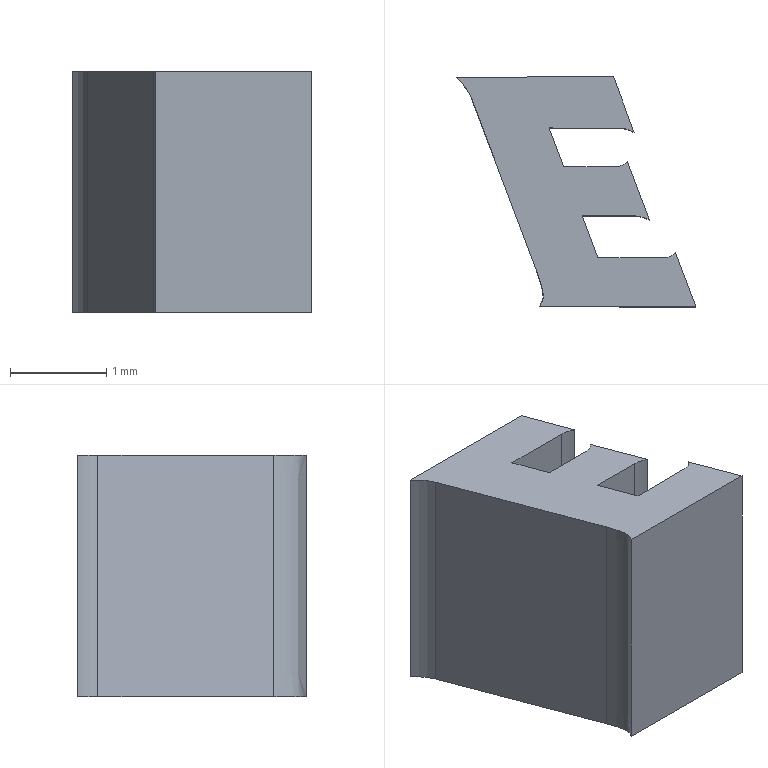Part | STEP file | lll_id1122_x_t | 1 solid | 20 faces | box 2.495 x 2.384 x 2.5 mm | volume 7.215 mm3 | plane 14 | cylinder 5 | other 1 | commonest cylinder face diameters 0.266 x1 0.267 x1 0.57 x1 0.572 x1 1.051 x1
STEP:
#1=CARTESIAN_POINT('',(394.185,-124.396,2.35));
#2=VERTEX_POINT('',#1);
#3=CARTESIAN_POINT('',(394.399,-124.962,2.35));
#4=VERTEX_POINT('',#3);
#5=CARTESIAN_POINT('',(394.187,-124.396,2.35));
#6=DIRECTION('',(0.3496,-0.9369,0.));
#7=VECTOR('',#6,1.);
#8=LINE('',#5,#7);
#9=EDGE_CURVE('',#2,#4,#8,.T.);
#10=ORIENTED_EDGE('',*,*,#9,.T.);
#11=CARTESIAN_POINT('',(394.399,-124.962,-0.15));
#12=VERTEX_POINT('',#11);
#13=CARTESIAN_POINT('',(394.399,-124.962,-0.15));
#14=DIRECTION('',(0.,0.,1.));
#15=VECTOR('',#14,1.);
#16=LINE('',#13,#15);
#17=EDGE_CURVE('',#12,#4,#16,.T.);
#18=ORIENTED_EDGE('',*,*,#17,.F.);
#19=CARTESIAN_POINT('',(394.185,-124.396,-0.15));
#20=VERTEX_POINT('',#19);
#21=CARTESIAN_POINT('',(394.187,-124.396,-0.15));
#22=DIRECTION('',(0.3496,-0.9369,0.));
#23=VECTOR('',#22,1.);
#24=LINE('',#21,#23);
#25=EDGE_CURVE('',#20,#12,#24,.T.);
#26=ORIENTED_EDGE('',*,*,#25,.F.);
#27=CARTESIAN_POINT('',(394.186,-124.391,-0.15));
#28=DIRECTION('',(0.,0.,1.));
#29=VECTOR('',#28,1.);
#30=LINE('',#27,#29);
#31=EDGE_CURVE('',#20,#2,#30,.T.);
#32=ORIENTED_EDGE('',*,*,#31,.T.);
#33=EDGE_LOOP('',(#10,#18,#26,#32));
#34=FACE_OUTER_BOUND('',#33,.T.);
#35=CARTESIAN_POINT('',(394.187,-124.396,-0.15));
#36=DIRECTION('',(-0.9369,-0.3496,0.));
#37=DIRECTION('',(-0.3496,0.9369,0.));
#38=AXIS2_PLACEMENT_3D('',#35,#36,#37);
#39=PLANE('',#38);
#40=ADVANCED_FACE('',(#34),#39,.F.);
#41=CARTESIAN_POINT('',(392.776,-124.959,2.35));
#42=VERTEX_POINT('',#41);
#43=CARTESIAN_POINT('',(394.399,-124.962,2.35));
#44=DIRECTION('',(-1.,0.,0.));
#45=VECTOR('',#44,1.);
#46=LINE('',#43,#45);
#47=EDGE_CURVE('',#4,#42,#46,.T.);
#48=ORIENTED_EDGE('',*,*,#47,.T.);
#49=CARTESIAN_POINT('',(392.776,-124.959,-0.15));
#50=VERTEX_POINT('',#49);
#51=CARTESIAN_POINT('',(392.771,-124.962,-0.15));
#52=DIRECTION('',(0.,0.,1.));
#53=VECTOR('',#52,1.);
#54=LINE('',#51,#53);
#55=EDGE_CURVE('',#50,#42,#54,.T.);
#56=ORIENTED_EDGE('',*,*,#55,.F.);
#57=CARTESIAN_POINT('',(394.399,-124.962,-0.15));
#58=DIRECTION('',(-1.,0.,0.));
#59=VECTOR('',#58,1.);
#60=LINE('',#57,#59);
#61=EDGE_CURVE('',#12,#50,#60,.T.);
#62=ORIENTED_EDGE('',*,*,#61,.F.);
#63=ORIENTED_EDGE('',*,*,#17,.T.);
#64=EDGE_LOOP('',(#48,#56,#62,#63));
#65=FACE_OUTER_BOUND('',#64,.T.);
#66=CARTESIAN_POINT('',(394.399,-124.962,-0.15));
#67=DIRECTION('',(0.,1.,0.));
#68=DIRECTION('',(0.,0.,1.));
#69=AXIS2_PLACEMENT_3D('',#66,#67,#68);
#70=PLANE('',#69);
#71=ADVANCED_FACE('',(#65),#70,.F.);
#72=CARTESIAN_POINT('',(392.756,-124.618,2.35));
#73=VERTEX_POINT('',#72);
#74=CARTESIAN_POINT('',(392.776,-124.956,2.35));
#75=CARTESIAN_POINT('',(392.78,-124.952,2.35));
#76=CARTESIAN_POINT('',(392.783,-124.947,2.35));
#77=CARTESIAN_POINT('',(392.801,-124.921,2.35));
#78=CARTESIAN_POINT('',(392.81,-124.897,2.35));
#79=CARTESIAN_POINT('',(392.814,-124.858,2.35));
#80=CARTESIAN_POINT('',(392.815,-124.845,2.35));
#81=CARTESIAN_POINT('',(392.813,-124.821,2.35));
#82=CARTESIAN_POINT('',(392.812,-124.81,2.35));
#83=CARTESIAN_POINT('',(392.808,-124.788,2.35));
#84=CARTESIAN_POINT('',(392.806,-124.777,2.35));
#85=CARTESIAN_POINT('',(392.8,-124.756,2.35));
#86=CARTESIAN_POINT('',(392.797,-124.745,2.35));
#87=CARTESIAN_POINT('',(392.787,-124.709,2.35));
#88=CARTESIAN_POINT('',(392.779,-124.685,2.35));
#89=CARTESIAN_POINT('',(392.766,-124.646,2.35));
#90=CARTESIAN_POINT('',(392.761,-124.632,2.35));
#91=CARTESIAN_POINT('',(392.756,-124.618,2.35));
#92=(BOUNDED_CURVE()B_SPLINE_CURVE(3,(#74,#75,#76,#77,#78,#79,#80,#81,#82,#83,#84,#85,#86,#87,#88,#89,#90,#91),.UNSPECIFIED.,.F.,.F.)B_SPLINE_CURVE_WITH_KNOTS((4,2,2,2,2,2,2,2,4),(0.,0.04796,0.2688,0.3781,0.4712,0.5646,0.6581,0.8756,1.),.UNSPECIFIED.)CURVE()GEOMETRIC_REPRESENTATION_ITEM()RATIONAL_B_SPLINE_CURVE((0.5002,0.4999,0.4999,0.4901,0.4901,0.4988,0.4988,0.4998,0.4998,0.5,0.5,0.5002,0.5002,0.5002,0.5002,0.5002,0.5002,0.5002))REPRESENTATION_ITEM(''));
#93=EDGE_CURVE('',#42,#73,#92,.T.);
#94=ORIENTED_EDGE('',*,*,#93,.T.);
#95=CARTESIAN_POINT('',(392.756,-124.618,-0.15));
#96=VERTEX_POINT('',#95);
#97=CARTESIAN_POINT('',(392.756,-124.618,-0.15));
#98=DIRECTION('',(0.,0.,1.));
#99=VECTOR('',#98,1.);
#100=LINE('',#97,#99);
#101=EDGE_CURVE('',#96,#73,#100,.T.);
#102=ORIENTED_EDGE('',*,*,#101,.F.);
#103=CARTESIAN_POINT('',(392.774,-124.959,-0.15));
#104=CARTESIAN_POINT('',(392.775,-124.958,-0.15));
#105=CARTESIAN_POINT('',(392.775,-124.957,-0.15));
#106=CARTESIAN_POINT('',(392.78,-124.952,-0.15));
#107=CARTESIAN_POINT('',(392.783,-124.947,-0.15));
#108=CARTESIAN_POINT('',(392.801,-124.921,-0.15));
#109=CARTESIAN_POINT('',(392.81,-124.897,-0.15));
#110=CARTESIAN_POINT('',(392.814,-124.858,-0.15));
#111=CARTESIAN_POINT('',(392.815,-124.845,-0.15));
#112=CARTESIAN_POINT('',(392.813,-124.821,-0.15));
#113=CARTESIAN_POINT('',(392.812,-124.81,-0.15));
#114=CARTESIAN_POINT('',(392.808,-124.788,-0.15));
#115=CARTESIAN_POINT('',(392.806,-124.777,-0.15));
#116=CARTESIAN_POINT('',(392.8,-124.756,-0.15));
#117=CARTESIAN_POINT('',(392.797,-124.745,-0.15));
#118=CARTESIAN_POINT('',(392.787,-124.709,-0.15));
#119=CARTESIAN_POINT('',(392.779,-124.685,-0.15));
#120=CARTESIAN_POINT('',(392.766,-124.646,-0.15));
#121=CARTESIAN_POINT('',(392.761,-124.632,-0.15));
#122=CARTESIAN_POINT('',(392.756,-124.618,-0.15));
#123=(BOUNDED_CURVE()B_SPLINE_CURVE(3,(#103,#104,#105,#106,#107,#108,#109,#110,#111,#112,#113,#114,#115,#116,#117,#118,#119,#120,#121,#122),.UNSPECIFIED.,.F.,.F.)B_SPLINE_CURVE_WITH_KNOTS((4,2,2,2,2,2,2,2,2,4),(0.,0.009901,0.05739,0.276,0.3843,0.4765,0.5689,0.6615,0.8769,1.),.UNSPECIFIED.)CURVE()GEOMETRIC_REPRESENTATION_ITEM()RATIONAL_B_SPLINE_CURVE((0.5002,0.5002,0.5002,0.4999,0.4999,0.4901,0.4901,0.4988,0.4988,0.4998,0.4998,0.5,0.5,0.5002,0.5002,0.5002,0.5002,0.5002,0.5002,0.5002))REPRESENTATION_ITEM(''));
#124=EDGE_CURVE('',#50,#96,#123,.T.);
#125=ORIENTED_EDGE('',*,*,#124,.F.);
#126=ORIENTED_EDGE('',*,*,#55,.T.);
#127=EDGE_LOOP('',(#94,#102,#125,#126));
#128=FACE_OUTER_BOUND('',#127,.T.);
#129=CARTESIAN_POINT('',(392.771,-124.962,-0.15));
#130=CARTESIAN_POINT('',(392.772,-124.961,-0.15));
#131=CARTESIAN_POINT('',(392.773,-124.96,-0.15));
#132=CARTESIAN_POINT('',(392.775,-124.958,-0.15));
#133=CARTESIAN_POINT('',(392.775,-124.957,-0.15));
#134=CARTESIAN_POINT('',(392.78,-124.952,-0.15));
#135=CARTESIAN_POINT('',(392.783,-124.947,-0.15));
#136=CARTESIAN_POINT('',(392.801,-124.921,-0.15));
#137=CARTESIAN_POINT('',(392.81,-124.897,-0.15));
#138=CARTESIAN_POINT('',(392.814,-124.858,-0.15));
#139=CARTESIAN_POINT('',(392.815,-124.845,-0.15));
#140=CARTESIAN_POINT('',(392.813,-124.821,-0.15));
#141=CARTESIAN_POINT('',(392.812,-124.81,-0.15));
#142=CARTESIAN_POINT('',(392.808,-124.788,-0.15));
#143=CARTESIAN_POINT('',(392.806,-124.777,-0.15));
#144=CARTESIAN_POINT('',(392.8,-124.756,-0.15));
#145=CARTESIAN_POINT('',(392.797,-124.745,-0.15));
#146=CARTESIAN_POINT('',(392.787,-124.709,-0.15));
#147=CARTESIAN_POINT('',(392.779,-124.685,-0.15));
#148=CARTESIAN_POINT('',(392.766,-124.646,-0.15));
#149=CARTESIAN_POINT('',(392.761,-124.632,-0.15));
#150=CARTESIAN_POINT('',(392.756,-124.618,-0.15));
#151=(BOUNDED_CURVE()B_SPLINE_CURVE(3,(#129,#130,#131,#132,#133,#134,#135,#136,#137,#138,#139,#140,#141,#142,#143,#144,#145,#146,#147,#148,#149,#150),.UNSPECIFIED.,.F.,.F.)B_SPLINE_CURVE_WITH_KNOTS((4,2,2,2,2,2,2,2,2,2,4),(0.,0.01065,0.02045,0.06743,0.2837,0.3908,0.4821,0.5735,0.6651,0.8782,1.),.UNSPECIFIED.)CURVE()GEOMETRIC_REPRESENTATION_ITEM()RATIONAL_B_SPLINE_CURVE((0.5002,0.5002,0.5002,0.5002,0.5002,0.4999,0.4999,0.4901,0.4901,0.4988,0.4988,0.4998,0.4998,0.5,0.5,0.5002,0.5002,0.5002,0.5002,0.5002,0.5002,0.5002))REPRESENTATION_ITEM(''));
#152=DIRECTION('',(0.,0.,1.));
#153=VECTOR('',#152,1.);
#154=SURFACE_OF_LINEAR_EXTRUSION('',#151,#153);
#155=ADVANCED_FACE('',(#128),#154,.F.);
#156=CARTESIAN_POINT('',(392.069,-122.793,2.35));
#157=VERTEX_POINT('',#156);
#158=CARTESIAN_POINT('',(392.756,-124.618,2.35));
#159=DIRECTION('',(-0.3523,0.9359,0.));
#160=VECTOR('',#159,1.);
#161=LINE('',#158,#160);
#162=EDGE_CURVE('',#73,#157,#161,.T.);
#163=ORIENTED_EDGE('',*,*,#162,.T.);
#164=CARTESIAN_POINT('',(392.069,-122.793,-0.15));
#165=VERTEX_POINT('',#164);
#166=CARTESIAN_POINT('',(392.069,-122.793,-0.15));
#167=DIRECTION('',(0.,0.,1.));
#168=VECTOR('',#167,1.);
#169=LINE('',#166,#168);
#170=EDGE_CURVE('',#165,#157,#169,.T.);
#171=ORIENTED_EDGE('',*,*,#170,.F.);
#172=CARTESIAN_POINT('',(392.756,-124.618,-0.15));
#173=DIRECTION('',(-0.3523,0.9359,0.));
#174=VECTOR('',#173,1.);
#175=LINE('',#172,#174);
#176=EDGE_CURVE('',#96,#165,#175,.T.);
#177=ORIENTED_EDGE('',*,*,#176,.F.);
#178=ORIENTED_EDGE('',*,*,#101,.T.);
#179=EDGE_LOOP('',(#163,#171,#177,#178));
#180=FACE_OUTER_BOUND('',#179,.T.);
#181=CARTESIAN_POINT('',(392.756,-124.618,-0.15));
#182=DIRECTION('',(0.9359,0.3523,0.));
#183=DIRECTION('',(0.3523,-0.9359,0.));
#184=AXIS2_PLACEMENT_3D('',#181,#182,#183);
#185=PLANE('',#184);
#186=ADVANCED_FACE('',(#180),#185,.F.);
#187=CARTESIAN_POINT('',(391.91,-122.58,2.35));
#188=VERTEX_POINT('',#187);
#189=CARTESIAN_POINT('',(391.583,-122.994,2.35));
#190=DIRECTION('',(0.,0.,1.));
#191=DIRECTION('',(-1.,0.,0.));
#192=AXIS2_PLACEMENT_3D('',#189,#190,#191);
#193=CIRCLE('',#192,0.5257);
#194=EDGE_CURVE('',#157,#188,#193,.T.);
#195=ORIENTED_EDGE('',*,*,#194,.T.);
#196=CARTESIAN_POINT('',(391.91,-122.58,-0.15));
#197=VERTEX_POINT('',#196);
#198=CARTESIAN_POINT('',(391.904,-122.578,-0.15));
#199=DIRECTION('',(0.,0.,1.));
#200=VECTOR('',#199,1.);
#201=LINE('',#198,#200);
#202=EDGE_CURVE('',#197,#188,#201,.T.);
#203=ORIENTED_EDGE('',*,*,#202,.F.);
#204=CARTESIAN_POINT('',(391.583,-122.994,-0.15));
#205=DIRECTION('',(0.,0.,1.));
#206=DIRECTION('',(-1.,0.,0.));
#207=AXIS2_PLACEMENT_3D('',#204,#205,#206);
#208=CIRCLE('',#207,0.5257);
#209=EDGE_CURVE('',#165,#197,#208,.T.);
#210=ORIENTED_EDGE('',*,*,#209,.F.);
#211=ORIENTED_EDGE('',*,*,#170,.T.);
#212=EDGE_LOOP('',(#195,#203,#210,#211));
#213=FACE_OUTER_BOUND('',#212,.T.);
#214=CARTESIAN_POINT('',(391.583,-122.994,-0.15));
#215=DIRECTION('',(0.,0.,1.));
#216=DIRECTION('',(1.,0.,0.));
#217=AXIS2_PLACEMENT_3D('',#214,#215,#216);
#218=CYLINDRICAL_SURFACE('',#217,0.5257);
#219=ADVANCED_FACE('',(#213),#218,.F.);
#220=CARTESIAN_POINT('',(393.544,-122.578,2.35));
#221=VERTEX_POINT('',#220);
#222=CARTESIAN_POINT('',(391.91,-122.578,2.35));
#223=DIRECTION('',(1.,0.,0.));
#224=VECTOR('',#223,1.);
#225=LINE('',#222,#224);
#226=EDGE_CURVE('',#188,#221,#225,.T.);
#227=ORIENTED_EDGE('',*,*,#226,.T.);
#228=CARTESIAN_POINT('',(393.544,-122.578,-0.15));
#229=VERTEX_POINT('',#228);
#230=CARTESIAN_POINT('',(393.544,-122.578,-0.15));
#231=DIRECTION('',(0.,0.,1.));
#232=VECTOR('',#231,1.);
#233=LINE('',#230,#232);
#234=EDGE_CURVE('',#229,#221,#233,.T.);
#235=ORIENTED_EDGE('',*,*,#234,.F.);
#236=CARTESIAN_POINT('',(391.91,-122.578,-0.15));
#237=DIRECTION('',(1.,0.,0.));
#238=VECTOR('',#237,1.);
#239=LINE('',#236,#238);
#240=EDGE_CURVE('',#197,#229,#239,.T.);
#241=ORIENTED_EDGE('',*,*,#240,.F.);
#242=ORIENTED_EDGE('',*,*,#202,.T.);
#243=EDGE_LOOP('',(#227,#235,#241,#242));
#244=FACE_OUTER_BOUND('',#243,.T.);
#245=CARTESIAN_POINT('',(391.91,-122.578,-0.15));
#246=DIRECTION('',(0.,-1.,0.));
#247=DIRECTION('',(0.,0.,-1.));
#248=AXIS2_PLACEMENT_3D('',#245,#246,#247);
#249=PLANE('',#248);
#250=ADVANCED_FACE('',(#244),#249,.F.);
#251=CARTESIAN_POINT('',(393.757,-123.151,2.35));
#252=VERTEX_POINT('',#251);
#253=CARTESIAN_POINT('',(393.544,-122.578,2.35));
#254=DIRECTION('',(0.3505,-0.9366,0.));
#255=VECTOR('',#254,1.);
#256=LINE('',#253,#255);
#257=EDGE_CURVE('',#221,#252,#256,.T.);
#258=ORIENTED_EDGE('',*,*,#257,.T.);
#259=CARTESIAN_POINT('',(393.757,-123.151,-0.15));
#260=VERTEX_POINT('',#259);
#261=CARTESIAN_POINT('',(393.761,-123.156,-0.15));
#262=DIRECTION('',(0.,0.,1.));
#263=VECTOR('',#262,1.);
#264=LINE('',#261,#263);
#265=EDGE_CURVE('',#260,#252,#264,.T.);
#266=ORIENTED_EDGE('',*,*,#265,.F.);
#267=CARTESIAN_POINT('',(393.544,-122.578,-0.15));
#268=DIRECTION('',(0.3505,-0.9366,0.));
#269=VECTOR('',#268,1.);
#270=LINE('',#267,#269);
#271=EDGE_CURVE('',#229,#260,#270,.T.);
#272=ORIENTED_EDGE('',*,*,#271,.F.);
#273=ORIENTED_EDGE('',*,*,#234,.T.);
#274=EDGE_LOOP('',(#258,#266,#272,#273));
#275=FACE_OUTER_BOUND('',#274,.T.);
#276=CARTESIAN_POINT('',(393.544,-122.578,-0.15));
#277=DIRECTION('',(-0.9366,-0.3505,0.));
#278=DIRECTION('',(-0.3505,0.9366,0.));
#279=AXIS2_PLACEMENT_3D('',#276,#277,#278);
#280=PLANE('',#279);
#281=ADVANCED_FACE('',(#275),#280,.F.);
#282=CARTESIAN_POINT('',(393.604,-123.11,2.35));
#283=VERTEX_POINT('',#282);
#284=CARTESIAN_POINT('',(393.606,-123.395,2.35));
#285=DIRECTION('',(0.,0.,1.));
#286=DIRECTION('',(-1.,0.,0.));
#287=AXIS2_PLACEMENT_3D('',#284,#285,#286);
#288=CIRCLE('',#287,0.2848);
#289=EDGE_CURVE('',#252,#283,#288,.T.);
#290=ORIENTED_EDGE('',*,*,#289,.T.);
#291=CARTESIAN_POINT('',(393.604,-123.11,-0.15));
#292=VERTEX_POINT('',#291);
#293=CARTESIAN_POINT('',(393.604,-123.11,-0.15));
#294=DIRECTION('',(0.,0.,1.));
#295=VECTOR('',#294,1.);
#296=LINE('',#293,#295);
#297=EDGE_CURVE('',#292,#283,#296,.T.);
#298=ORIENTED_EDGE('',*,*,#297,.F.);
#299=CARTESIAN_POINT('',(393.606,-123.395,-0.15));
#300=DIRECTION('',(0.,0.,1.));
#301=DIRECTION('',(-1.,0.,0.));
#302=AXIS2_PLACEMENT_3D('',#299,#300,#301);
#303=CIRCLE('',#302,0.2848);
#304=EDGE_CURVE('',#260,#292,#303,.T.);
#305=ORIENTED_EDGE('',*,*,#304,.F.);
#306=ORIENTED_EDGE('',*,*,#265,.T.);
#307=EDGE_LOOP('',(#290,#298,#305,#306));
#308=FACE_OUTER_BOUND('',#307,.T.);
#309=CARTESIAN_POINT('',(393.606,-123.395,-0.15));
#310=DIRECTION('',(0.,0.,1.));
#311=DIRECTION('',(1.,0.,0.));
#312=AXIS2_PLACEMENT_3D('',#309,#310,#311);
#313=CYLINDRICAL_SURFACE('',#312,0.2848);
#314=ADVANCED_FACE('',(#308),#313,.F.);
#315=CARTESIAN_POINT('',(392.877,-123.108,2.35));
#316=VERTEX_POINT('',#315);
#317=CARTESIAN_POINT('',(393.604,-123.11,2.35));
#318=DIRECTION('',(-1.,0.003072,0.));
#319=VECTOR('',#318,1.);
#320=LINE('',#317,#319);
#321=EDGE_CURVE('',#283,#316,#320,.T.);
#322=ORIENTED_EDGE('',*,*,#321,.T.);
#323=CARTESIAN_POINT('',(392.877,-123.108,-0.15));
#324=VERTEX_POINT('',#323);
#325=CARTESIAN_POINT('',(392.877,-123.108,-0.15));
#326=DIRECTION('',(0.,0.,1.));
#327=VECTOR('',#326,1.);
#328=LINE('',#325,#327);
#329=EDGE_CURVE('',#324,#316,#328,.T.);
#330=ORIENTED_EDGE('',*,*,#329,.F.);
#331=CARTESIAN_POINT('',(393.604,-123.11,-0.15));
#332=DIRECTION('',(-1.,0.003072,0.));
#333=VECTOR('',#332,1.);
#334=LINE('',#331,#333);
#335=EDGE_CURVE('',#292,#324,#334,.T.);
#336=ORIENTED_EDGE('',*,*,#335,.F.);
#337=ORIENTED_EDGE('',*,*,#297,.T.);
#338=EDGE_LOOP('',(#322,#330,#336,#337));
#339=FACE_OUTER_BOUND('',#338,.T.);
#340=CARTESIAN_POINT('',(393.604,-123.11,-0.15));
#341=DIRECTION('',(0.003072,1.,0.));
#342=DIRECTION('',(1.,-0.003072,0.));
#343=AXIS2_PLACEMENT_3D('',#340,#341,#342);
#344=PLANE('',#343);
#345=ADVANCED_FACE('',(#339),#344,.F.);
#346=CARTESIAN_POINT('',(393.027,-123.51,2.35));
#347=VERTEX_POINT('',#346);
#348=CARTESIAN_POINT('',(392.877,-123.108,2.35));
#349=DIRECTION('',(0.3491,-0.9371,0.));
#350=VECTOR('',#349,1.);
#351=LINE('',#348,#350);
#352=EDGE_CURVE('',#316,#347,#351,.T.);
#353=ORIENTED_EDGE('',*,*,#352,.T.);
#354=CARTESIAN_POINT('',(393.027,-123.51,-0.15));
#355=VERTEX_POINT('',#354);
#356=CARTESIAN_POINT('',(393.027,-123.51,-0.15));
#357=DIRECTION('',(0.,0.,1.));
#358=VECTOR('',#357,1.);
#359=LINE('',#356,#358);
#360=EDGE_CURVE('',#355,#347,#359,.T.);
#361=ORIENTED_EDGE('',*,*,#360,.F.);
#362=CARTESIAN_POINT('',(392.877,-123.108,-0.15));
#363=DIRECTION('',(0.3491,-0.9371,0.));
#364=VECTOR('',#363,1.);
#365=LINE('',#362,#364);
#366=EDGE_CURVE('',#324,#355,#365,.T.);
#367=ORIENTED_EDGE('',*,*,#366,.F.);
#368=ORIENTED_EDGE('',*,*,#329,.T.);
#369=EDGE_LOOP('',(#353,#361,#367,#368));
#370=FACE_OUTER_BOUND('',#369,.T.);
#371=CARTESIAN_POINT('',(392.877,-123.108,-0.15));
#372=DIRECTION('',(-0.9371,-0.3491,0.));
#373=DIRECTION('',(-0.3491,0.9371,0.));
#374=AXIS2_PLACEMENT_3D('',#371,#372,#373);
#375=PLANE('',#374);
#376=ADVANCED_FACE('',(#370),#375,.F.);
#377=CARTESIAN_POINT('',(393.573,-123.507,2.35));
#378=VERTEX_POINT('',#377);
#379=CARTESIAN_POINT('',(393.027,-123.51,2.35));
#380=DIRECTION('',(1.,0.006653,0.));
#381=VECTOR('',#380,1.);
#382=LINE('',#379,#381);
#383=EDGE_CURVE('',#347,#378,#382,.T.);
#384=ORIENTED_EDGE('',*,*,#383,.T.);
#385=CARTESIAN_POINT('',(393.573,-123.507,-0.15));
#386=VERTEX_POINT('',#385);
#387=CARTESIAN_POINT('',(393.573,-123.507,-0.15));
#388=DIRECTION('',(0.,0.,1.));
#389=VECTOR('',#388,1.);
#390=LINE('',#387,#389);
#391=EDGE_CURVE('',#386,#378,#390,.T.);
#392=ORIENTED_EDGE('',*,*,#391,.F.);
#393=CARTESIAN_POINT('',(393.027,-123.51,-0.15));
#394=DIRECTION('',(1.,0.006653,0.));
#395=VECTOR('',#394,1.);
#396=LINE('',#393,#395);
#397=EDGE_CURVE('',#355,#386,#396,.T.);
#398=ORIENTED_EDGE('',*,*,#397,.F.);
#399=ORIENTED_EDGE('',*,*,#360,.T.);
#400=EDGE_LOOP('',(#384,#392,#398,#399));
#401=FACE_OUTER_BOUND('',#400,.T.);
#402=CARTESIAN_POINT('',(393.027,-123.51,-0.15));
#403=DIRECTION('',(0.006653,-1.,0.));
#404=DIRECTION('',(-1.,-0.006653,0.));
#405=AXIS2_PLACEMENT_3D('',#402,#403,#404);
#406=PLANE('',#405);
#407=ADVANCED_FACE('',(#401),#406,.F.);
#408=CARTESIAN_POINT('',(393.687,-123.452,2.35));
#409=VERTEX_POINT('',#408);
#410=CARTESIAN_POINT('',(393.576,-123.374,2.35));
#411=DIRECTION('',(0.,0.,1.));
#412=DIRECTION('',(-1.,0.,0.));
#413=AXIS2_PLACEMENT_3D('',#410,#411,#412);
#414=CIRCLE('',#413,0.1333);
#415=EDGE_CURVE('',#378,#409,#414,.T.);
#416=ORIENTED_EDGE('',*,*,#415,.T.);
#417=CARTESIAN_POINT('',(393.687,-123.452,-0.15));
#418=VERTEX_POINT('',#417);
#419=CARTESIAN_POINT('',(393.687,-123.447,-0.15));
#420=DIRECTION('',(0.,0.,1.));
#421=VECTOR('',#420,1.);
#422=LINE('',#419,#421);
#423=EDGE_CURVE('',#418,#409,#422,.T.);
#424=ORIENTED_EDGE('',*,*,#423,.F.);
#425=CARTESIAN_POINT('',(393.576,-123.374,-0.15));
#426=DIRECTION('',(0.,0.,1.));
#427=DIRECTION('',(-1.,0.,0.));
#428=AXIS2_PLACEMENT_3D('',#425,#426,#427);
#429=CIRCLE('',#428,0.1333);
#430=EDGE_CURVE('',#386,#418,#429,.T.);
#431=ORIENTED_EDGE('',*,*,#430,.F.);
#432=ORIENTED_EDGE('',*,*,#391,.T.);
#433=EDGE_LOOP('',(#416,#424,#431,#432));
#434=FACE_OUTER_BOUND('',#433,.T.);
#435=CARTESIAN_POINT('',(393.576,-123.374,-0.15));
#436=DIRECTION('',(0.,0.,1.));
#437=DIRECTION('',(1.,0.,0.));
#438=AXIS2_PLACEMENT_3D('',#435,#436,#437);
#439=CYLINDRICAL_SURFACE('',#438,0.1333);
#440=ADVANCED_FACE('',(#434),#439,.F.);
#441=CARTESIAN_POINT('',(393.915,-124.061,2.35));
#442=VERTEX_POINT('',#441);
#443=CARTESIAN_POINT('',(393.689,-123.452,2.35));
#444=DIRECTION('',(0.3508,-0.9364,0.));
#445=VECTOR('',#444,1.);
#446=LINE('',#443,#445);
#447=EDGE_CURVE('',#409,#442,#446,.T.);
#448=ORIENTED_EDGE('',*,*,#447,.T.);
#449=CARTESIAN_POINT('',(393.915,-124.061,-0.15));
#450=VERTEX_POINT('',#449);
#451=CARTESIAN_POINT('',(393.919,-124.066,-0.15));
#452=DIRECTION('',(0.,0.,1.));
#453=VECTOR('',#452,1.);
#454=LINE('',#451,#453);
#455=EDGE_CURVE('',#450,#442,#454,.T.);
#456=ORIENTED_EDGE('',*,*,#455,.F.);
#457=CARTESIAN_POINT('',(393.689,-123.452,-0.15));
#458=DIRECTION('',(0.3508,-0.9364,0.));
#459=VECTOR('',#458,1.);
#460=LINE('',#457,#459);
#461=EDGE_CURVE('',#418,#450,#460,.T.);
#462=ORIENTED_EDGE('',*,*,#461,.F.);
#463=ORIENTED_EDGE('',*,*,#423,.T.);
#464=EDGE_LOOP('',(#448,#456,#462,#463));
#465=FACE_OUTER_BOUND('',#464,.T.);
#466=CARTESIAN_POINT('',(393.689,-123.452,-0.15));
#467=DIRECTION('',(-0.9364,-0.3508,0.));
#468=DIRECTION('',(-0.3508,0.9364,0.));
#469=AXIS2_PLACEMENT_3D('',#466,#467,#468);
#470=PLANE('',#469);
#471=ADVANCED_FACE('',(#465),#470,.F.);
#472=CARTESIAN_POINT('',(393.762,-124.02,2.35));
#473=VERTEX_POINT('',#472);
#474=CARTESIAN_POINT('',(393.764,-124.306,2.35));
#475=DIRECTION('',(0.,0.,1.));
#476=DIRECTION('',(-1.,0.,0.));
#477=AXIS2_PLACEMENT_3D('',#474,#475,#476);
#478=CIRCLE('',#477,0.2859);
#479=EDGE_CURVE('',#442,#473,#478,.T.);
#480=ORIENTED_EDGE('',*,*,#479,.T.);
#481=CARTESIAN_POINT('',(393.762,-124.02,-0.15));
#482=VERTEX_POINT('',#481);
#483=CARTESIAN_POINT('',(393.762,-124.02,-0.15));
#484=DIRECTION('',(0.,0.,1.));
#485=VECTOR('',#484,1.);
#486=LINE('',#483,#485);
#487=EDGE_CURVE('',#482,#473,#486,.T.);
#488=ORIENTED_EDGE('',*,*,#487,.F.);
#489=CARTESIAN_POINT('',(393.764,-124.306,-0.15));
#490=DIRECTION('',(0.,0.,1.));
#491=DIRECTION('',(-1.,0.,0.));
#492=AXIS2_PLACEMENT_3D('',#489,#490,#491);
#493=CIRCLE('',#492,0.2859);
#494=EDGE_CURVE('',#450,#482,#493,.T.);
#495=ORIENTED_EDGE('',*,*,#494,.F.);
#496=ORIENTED_EDGE('',*,*,#455,.T.);
#497=EDGE_LOOP('',(#480,#488,#495,#496));
#498=FACE_OUTER_BOUND('',#497,.T.);
#499=CARTESIAN_POINT('',(393.764,-124.306,-0.15));
#500=DIRECTION('',(0.,0.,1.));
#501=DIRECTION('',(1.,0.,0.));
#502=AXIS2_PLACEMENT_3D('',#499,#500,#501);
#503=CYLINDRICAL_SURFACE('',#502,0.2859);
#504=ADVANCED_FACE('',(#498),#503,.F.);
#505=CARTESIAN_POINT('',(393.217,-124.018,2.35));
#506=VERTEX_POINT('',#505);
#507=CARTESIAN_POINT('',(393.762,-124.02,2.35));
#508=DIRECTION('',(-1.,0.004114,0.));
#509=VECTOR('',#508,1.);
#510=LINE('',#507,#509);
#511=EDGE_CURVE('',#473,#506,#510,.T.);
#512=ORIENTED_EDGE('',*,*,#511,.T.);
#513=CARTESIAN_POINT('',(393.217,-124.018,-0.15));
#514=VERTEX_POINT('',#513);
#515=CARTESIAN_POINT('',(393.217,-124.018,-0.15));
#516=DIRECTION('',(0.,0.,1.));
#517=VECTOR('',#516,1.);
#518=LINE('',#515,#517);
#519=EDGE_CURVE('',#514,#506,#518,.T.);
#520=ORIENTED_EDGE('',*,*,#519,.F.);
#521=CARTESIAN_POINT('',(393.762,-124.02,-0.15));
#522=DIRECTION('',(-1.,0.004114,0.));
#523=VECTOR('',#522,1.);
#524=LINE('',#521,#523);
#525=EDGE_CURVE('',#482,#514,#524,.T.);
#526=ORIENTED_EDGE('',*,*,#525,.F.);
#527=ORIENTED_EDGE('',*,*,#487,.T.);
#528=EDGE_LOOP('',(#512,#520,#526,#527));
#529=FACE_OUTER_BOUND('',#528,.T.);
#530=CARTESIAN_POINT('',(393.762,-124.02,-0.15));
#531=DIRECTION('',(0.004114,1.,0.));
#532=DIRECTION('',(1.,-0.004114,0.));
#533=AXIS2_PLACEMENT_3D('',#530,#531,#532);
#534=PLANE('',#533);
#535=ADVANCED_FACE('',(#529),#534,.F.);
#536=CARTESIAN_POINT('',(393.38,-124.455,2.35));
#537=VERTEX_POINT('',#536);
#538=CARTESIAN_POINT('',(393.217,-124.018,2.35));
#539=DIRECTION('',(0.3507,-0.9365,0.));
#540=VECTOR('',#539,1.);
#541=LINE('',#538,#540);
#542=EDGE_CURVE('',#506,#537,#541,.T.);
#543=ORIENTED_EDGE('',*,*,#542,.T.);
#544=CARTESIAN_POINT('',(393.38,-124.455,-0.15));
#545=VERTEX_POINT('',#544);
#546=CARTESIAN_POINT('',(393.38,-124.455,-0.15));
#547=DIRECTION('',(0.,0.,1.));
#548=VECTOR('',#547,1.);
#549=LINE('',#546,#548);
#550=EDGE_CURVE('',#545,#537,#549,.T.);
#551=ORIENTED_EDGE('',*,*,#550,.F.);
#552=CARTESIAN_POINT('',(393.217,-124.018,-0.15));
#553=DIRECTION('',(0.3507,-0.9365,0.));
#554=VECTOR('',#553,1.);
#555=LINE('',#552,#554);
#556=EDGE_CURVE('',#514,#545,#555,.T.);
#557=ORIENTED_EDGE('',*,*,#556,.F.);
#558=ORIENTED_EDGE('',*,*,#519,.T.);
#559=EDGE_LOOP('',(#543,#551,#557,#558));
#560=FACE_OUTER_BOUND('',#559,.T.);
#561=CARTESIAN_POINT('',(393.217,-124.018,-0.15));
#562=DIRECTION('',(-0.9365,-0.3507,0.));
#563=DIRECTION('',(-0.3507,0.9365,0.));
#564=AXIS2_PLACEMENT_3D('',#561,#562,#563);
#565=PLANE('',#564);
#566=ADVANCED_FACE('',(#560),#565,.F.);
#567=CARTESIAN_POINT('',(394.072,-124.451,2.35));
#568=VERTEX_POINT('',#567);
#569=CARTESIAN_POINT('',(393.38,-124.455,2.35));
#570=DIRECTION('',(1.,0.005261,0.));
#571=VECTOR('',#570,1.);
#572=LINE('',#569,#571);
#573=EDGE_CURVE('',#537,#568,#572,.T.);
#574=ORIENTED_EDGE('',*,*,#573,.T.);
#575=CARTESIAN_POINT('',(394.072,-124.451,-0.15));
#576=VERTEX_POINT('',#575);
#577=CARTESIAN_POINT('',(394.072,-124.451,-0.15));
#578=DIRECTION('',(0.,0.,1.));
#579=VECTOR('',#578,1.);
#580=LINE('',#577,#579);
#581=EDGE_CURVE('',#576,#568,#580,.T.);
#582=ORIENTED_EDGE('',*,*,#581,.F.);
#583=CARTESIAN_POINT('',(393.38,-124.455,-0.15));
#584=DIRECTION('',(1.,0.005261,0.));
#585=VECTOR('',#584,1.);
#586=LINE('',#583,#585);
#587=EDGE_CURVE('',#545,#576,#586,.T.);
#588=ORIENTED_EDGE('',*,*,#587,.F.);
#589=ORIENTED_EDGE('',*,*,#550,.T.);
#590=EDGE_LOOP('',(#574,#582,#588,#589));
#591=FACE_OUTER_BOUND('',#590,.T.);
#592=CARTESIAN_POINT('',(393.38,-124.455,-0.15));
#593=DIRECTION('',(0.005261,-1.,0.));
#594=DIRECTION('',(-1.,-0.005261,0.));
#595=AXIS2_PLACEMENT_3D('',#592,#593,#594);
#596=PLANE('',#595);
#597=ADVANCED_FACE('',(#591),#596,.F.);
#598=CARTESIAN_POINT('',(394.074,-124.318,2.35));
#599=DIRECTION('',(0.,0.,1.));
#600=DIRECTION('',(-1.,0.,0.));
#601=AXIS2_PLACEMENT_3D('',#598,#599,#600);
#602=CIRCLE('',#601,0.1332);
#603=EDGE_CURVE('',#568,#2,#602,.T.);
#604=ORIENTED_EDGE('',*,*,#603,.T.);
#605=ORIENTED_EDGE('',*,*,#31,.F.);
#606=CARTESIAN_POINT('',(394.074,-124.318,-0.15));
#607=DIRECTION('',(0.,0.,1.));
#608=DIRECTION('',(-1.,0.,0.));
#609=AXIS2_PLACEMENT_3D('',#606,#607,#608);
#610=CIRCLE('',#609,0.1332);
#611=EDGE_CURVE('',#576,#20,#610,.T.);
#612=ORIENTED_EDGE('',*,*,#611,.F.);
#613=ORIENTED_EDGE('',*,*,#581,.T.);
#614=EDGE_LOOP('',(#604,#605,#612,#613));
#615=FACE_OUTER_BOUND('',#614,.T.);
#616=CARTESIAN_POINT('',(394.074,-124.318,-0.15));
#617=DIRECTION('',(0.,0.,1.));
#618=DIRECTION('',(1.,0.,0.));
#619=AXIS2_PLACEMENT_3D('',#616,#617,#618);
#620=CYLINDRICAL_SURFACE('',#619,0.1332);
#621=ADVANCED_FACE('',(#615),#620,.F.);
#622=ORIENTED_EDGE('',*,*,#25,.T.);
#623=ORIENTED_EDGE('',*,*,#61,.T.);
#624=ORIENTED_EDGE('',*,*,#124,.T.);
#625=ORIENTED_EDGE('',*,*,#176,.T.);
#626=ORIENTED_EDGE('',*,*,#209,.T.);
#627=ORIENTED_EDGE('',*,*,#240,.T.);
#628=ORIENTED_EDGE('',*,*,#271,.T.);
#629=ORIENTED_EDGE('',*,*,#304,.T.);
#630=ORIENTED_EDGE('',*,*,#335,.T.);
#631=ORIENTED_EDGE('',*,*,#366,.T.);
#632=ORIENTED_EDGE('',*,*,#397,.T.);
#633=ORIENTED_EDGE('',*,*,#430,.T.);
#634=ORIENTED_EDGE('',*,*,#461,.T.);
#635=ORIENTED_EDGE('',*,*,#494,.T.);
#636=ORIENTED_EDGE('',*,*,#525,.T.);
#637=ORIENTED_EDGE('',*,*,#556,.T.);
#638=ORIENTED_EDGE('',*,*,#587,.T.);
#639=ORIENTED_EDGE('',*,*,#611,.T.);
#640=EDGE_LOOP('',(#622,#623,#624,#625,#626,#627,#628,#629,#630,#631,#632,#633,#634,#635,#636,#637,#638,#639));
#641=FACE_OUTER_BOUND('',#640,.T.);
#642=CARTESIAN_POINT('',(392.808,-124.789,-0.15));
#643=DIRECTION('',(0.,0.,-1.));
#644=DIRECTION('',(-1.,0.,0.));
#645=AXIS2_PLACEMENT_3D('',#642,#643,#644);
#646=PLANE('',#645);
#647=ADVANCED_FACE('',(#641),#646,.T.);
#648=ORIENTED_EDGE('',*,*,#9,.F.);
#649=ORIENTED_EDGE('',*,*,#603,.F.);
#650=ORIENTED_EDGE('',*,*,#573,.F.);
#651=ORIENTED_EDGE('',*,*,#542,.F.);
#652=ORIENTED_EDGE('',*,*,#511,.F.);
#653=ORIENTED_EDGE('',*,*,#479,.F.);
#654=ORIENTED_EDGE('',*,*,#447,.F.);
#655=ORIENTED_EDGE('',*,*,#415,.F.);
#656=ORIENTED_EDGE('',*,*,#383,.F.);
#657=ORIENTED_EDGE('',*,*,#352,.F.);
#658=ORIENTED_EDGE('',*,*,#321,.F.);
#659=ORIENTED_EDGE('',*,*,#289,.F.);
#660=ORIENTED_EDGE('',*,*,#257,.F.);
#661=ORIENTED_EDGE('',*,*,#226,.F.);
#662=ORIENTED_EDGE('',*,*,#194,.F.);
#663=ORIENTED_EDGE('',*,*,#162,.F.);
#664=ORIENTED_EDGE('',*,*,#93,.F.);
#665=ORIENTED_EDGE('',*,*,#47,.F.);
#666=EDGE_LOOP('',(#648,#649,#650,#651,#652,#653,#654,#655,#656,#657,#658,#659,#660,#661,#662,#663,#664,#665));
#667=FACE_OUTER_BOUND('',#666,.T.);
#668=CARTESIAN_POINT('',(392.808,-124.789,2.35));
#669=DIRECTION('',(0.,0.,-1.));
#670=DIRECTION('',(-1.,0.,0.));
#671=AXIS2_PLACEMENT_3D('',#668,#669,#670);
#672=PLANE('',#671);
#673=ADVANCED_FACE('',(#667),#672,.F.);
#674=CLOSED_SHELL('',(#40,#71,#155,#186,#219,#250,#281,#314,#345,#376,#407,#440,#471,#504,#535,#566,#597,#621,#647,#673));
#675=MANIFOLD_SOLID_BREP('',#674);
#676=(LENGTH_UNIT()NAMED_UNIT(*)SI_UNIT(.MILLI.,.METRE.));
#677=UNCERTAINTY_MEASURE_WITH_UNIT(LENGTH_MEASURE(0.01401),#676,'','');
#678=(NAMED_UNIT(*)PLANE_ANGLE_UNIT()SI_UNIT($,.RADIAN.));
#679=PLANE_ANGLE_MEASURE_WITH_UNIT(PLANE_ANGLE_MEASURE(0.01745),#678);
#680=DIMENSIONAL_EXPONENTS(0.,0.,0.,0.,0.,0.,0.);
#681=(CONVERSION_BASED_UNIT('DEGREE',#679)NAMED_UNIT(#680)PLANE_ANGLE_UNIT());
#682=(NAMED_UNIT(*)SI_UNIT($,.STERADIAN.)SOLID_ANGLE_UNIT());
#683=(GEOMETRIC_REPRESENTATION_CONTEXT(3)GLOBAL_UNCERTAINTY_ASSIGNED_CONTEXT((#677))GLOBAL_UNIT_ASSIGNED_CONTEXT((#676,#681,#682))REPRESENTATION_CONTEXT('',''));
#684=ADVANCED_BREP_SHAPE_REPRESENTATION('',(#675),#683);